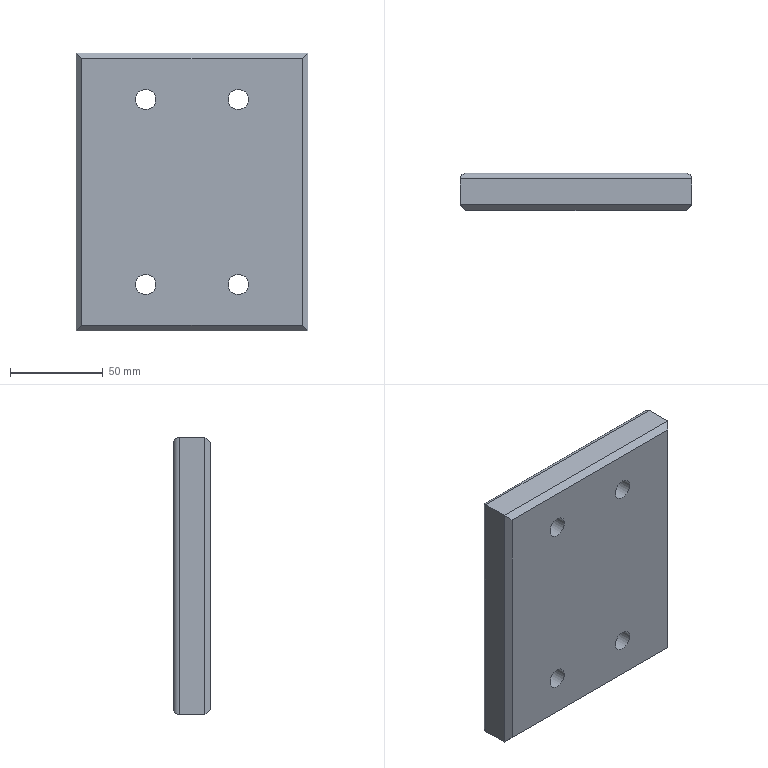Part | NX | features solid 2 | 1 solid | 26 faces | box 125 x 20 x 150 mm | volume 356923 mm3 | plane 14 | cylinder 12 | commonest cylinder face diameters 6 x4 11 x4 17.5 x4
STEP:
#1=CARTESIAN_POINT('',(-495.,793.,50.));
#2=VERTEX_POINT('',#1);
#3=CARTESIAN_POINT('',(-495.,807.,50.));
#4=VERTEX_POINT('',#3);
#5=CARTESIAN_POINT('',(-495.,790.,50.));
#6=DIRECTION('',(0.,1.,0.));
#7=VECTOR('',#6,1000.);
#8=LINE('',#5,#7);
#9=EDGE_CURVE('',#2,#4,#8,.T.);
#10=ORIENTED_EDGE('',*,*,#9,.F.);
#11=CARTESIAN_POINT('',(-620.,793.,50.));
#12=VERTEX_POINT('',#11);
#13=CARTESIAN_POINT('',(-620.,793.,50.));
#14=DIRECTION('',(-1.,0.,0.));
#15=VECTOR('',#14,1000.);
#16=LINE('',#13,#15);
#17=EDGE_CURVE('',#2,#12,#16,.T.);
#18=ORIENTED_EDGE('',*,*,#17,.T.);
#19=CARTESIAN_POINT('',(-620.,807.,50.));
#20=VERTEX_POINT('',#19);
#21=CARTESIAN_POINT('',(-620.,790.,50.));
#22=DIRECTION('',(0.,1.,0.));
#23=VECTOR('',#22,1000.);
#24=LINE('',#21,#23);
#25=EDGE_CURVE('',#12,#20,#24,.T.);
#26=ORIENTED_EDGE('',*,*,#25,.T.);
#27=CARTESIAN_POINT('',(-495.,807.,50.));
#28=DIRECTION('',(1.,0.,0.));
#29=VECTOR('',#28,1000.);
#30=LINE('',#27,#29);
#31=EDGE_CURVE('',#20,#4,#30,.T.);
#32=ORIENTED_EDGE('',*,*,#31,.T.);
#33=EDGE_LOOP('',(#10,#18,#26,#32));
#34=FACE_BOUND('',#33,.T.);
#35=CARTESIAN_POINT('',(-620.,790.,50.));
#36=DIRECTION('',(0.,0.,1.));
#37=DIRECTION('',(-1.,0.,0.));
#38=AXIS2_PLACEMENT_3D('',#35,#36,#37);
#39=PLANE('',#38);
#40=ADVANCED_FACE('',(#34),#39,.F.);
#41=CARTESIAN_POINT('',(-495.,793.,200.));
#42=VERTEX_POINT('',#41);
#43=CARTESIAN_POINT('',(-495.,807.,200.));
#44=VERTEX_POINT('',#43);
#45=CARTESIAN_POINT('',(-495.,790.,200.));
#46=DIRECTION('',(0.,1.,0.));
#47=VECTOR('',#46,1000.);
#48=LINE('',#45,#47);
#49=EDGE_CURVE('',#42,#44,#48,.T.);
#50=ORIENTED_EDGE('',*,*,#49,.F.);
#51=CARTESIAN_POINT('',(-495.,793.,50.));
#52=DIRECTION('',(0.,0.,-1.));
#53=VECTOR('',#52,1000.);
#54=LINE('',#51,#53);
#55=EDGE_CURVE('',#42,#2,#54,.T.);
#56=ORIENTED_EDGE('',*,*,#55,.T.);
#57=ORIENTED_EDGE('',*,*,#9,.T.);
#58=CARTESIAN_POINT('',(-495.,807.,200.));
#59=DIRECTION('',(0.,0.,1.));
#60=VECTOR('',#59,1000.);
#61=LINE('',#58,#60);
#62=EDGE_CURVE('',#4,#44,#61,.T.);
#63=ORIENTED_EDGE('',*,*,#62,.T.);
#64=EDGE_LOOP('',(#50,#56,#57,#63));
#65=FACE_BOUND('',#64,.T.);
#66=CARTESIAN_POINT('',(-495.,790.,50.));
#67=DIRECTION('',(-1.,0.,0.));
#68=DIRECTION('',(0.,-1.,0.));
#69=AXIS2_PLACEMENT_3D('',#66,#67,#68);
#70=PLANE('',#69);
#71=ADVANCED_FACE('',(#65),#70,.F.);
#72=CARTESIAN_POINT('',(-620.,793.,200.));
#73=VERTEX_POINT('',#72);
#74=CARTESIAN_POINT('',(-620.,807.,200.));
#75=VERTEX_POINT('',#74);
#76=CARTESIAN_POINT('',(-620.,790.,200.));
#77=DIRECTION('',(0.,1.,0.));
#78=VECTOR('',#77,1000.);
#79=LINE('',#76,#78);
#80=EDGE_CURVE('',#73,#75,#79,.T.);
#81=ORIENTED_EDGE('',*,*,#80,.F.);
#82=CARTESIAN_POINT('',(-495.,793.,200.));
#83=DIRECTION('',(1.,0.,0.));
#84=VECTOR('',#83,1000.);
#85=LINE('',#82,#84);
#86=EDGE_CURVE('',#73,#42,#85,.T.);
#87=ORIENTED_EDGE('',*,*,#86,.T.);
#88=ORIENTED_EDGE('',*,*,#49,.T.);
#89=CARTESIAN_POINT('',(-620.,807.,200.));
#90=DIRECTION('',(-1.,0.,0.));
#91=VECTOR('',#90,1000.);
#92=LINE('',#89,#91);
#93=EDGE_CURVE('',#44,#75,#92,.T.);
#94=ORIENTED_EDGE('',*,*,#93,.T.);
#95=EDGE_LOOP('',(#81,#87,#88,#94));
#96=FACE_BOUND('',#95,.T.);
#97=CARTESIAN_POINT('',(-495.,790.,200.));
#98=DIRECTION('',(0.,0.,-1.));
#99=DIRECTION('',(0.,-1.,0.));
#100=AXIS2_PLACEMENT_3D('',#97,#98,#99);
#101=PLANE('',#100);
#102=ADVANCED_FACE('',(#96),#101,.F.);
#103=ORIENTED_EDGE('',*,*,#25,.F.);
#104=CARTESIAN_POINT('',(-620.,793.,200.));
#105=DIRECTION('',(0.,0.,1.));
#106=VECTOR('',#105,1000.);
#107=LINE('',#104,#106);
#108=EDGE_CURVE('',#12,#73,#107,.T.);
#109=ORIENTED_EDGE('',*,*,#108,.T.);
#110=ORIENTED_EDGE('',*,*,#80,.T.);
#111=CARTESIAN_POINT('',(-620.,807.,50.));
#112=DIRECTION('',(0.,0.,-1.));
#113=VECTOR('',#112,1000.);
#114=LINE('',#111,#113);
#115=EDGE_CURVE('',#75,#20,#114,.T.);
#116=ORIENTED_EDGE('',*,*,#115,.T.);
#117=EDGE_LOOP('',(#103,#109,#110,#116));
#118=FACE_BOUND('',#117,.T.);
#119=CARTESIAN_POINT('',(-620.,790.,200.));
#120=DIRECTION('',(1.,0.,0.));
#121=DIRECTION('',(0.,0.,1.));
#122=AXIS2_PLACEMENT_3D('',#119,#120,#121);
#123=PLANE('',#122);
#124=ADVANCED_FACE('',(#118),#123,.F.);
#125=CARTESIAN_POINT('',(-498.,790.,53.));
#126=VERTEX_POINT('',#125);
#127=CARTESIAN_POINT('',(-498.,790.,197.));
#128=VERTEX_POINT('',#127);
#129=CARTESIAN_POINT('',(-498.,790.,50.));
#130=DIRECTION('',(0.,0.,1.));
#131=VECTOR('',#130,1000.);
#132=LINE('',#129,#131);
#133=EDGE_CURVE('',#126,#128,#132,.T.);
#134=ORIENTED_EDGE('',*,*,#133,.T.);
#135=CARTESIAN_POINT('',(-617.,790.,197.));
#136=VERTEX_POINT('',#135);
#137=CARTESIAN_POINT('',(-620.,790.,197.));
#138=DIRECTION('',(-1.,0.,0.));
#139=VECTOR('',#138,1000.);
#140=LINE('',#137,#139);
#141=EDGE_CURVE('',#128,#136,#140,.T.);
#142=ORIENTED_EDGE('',*,*,#141,.T.);
#143=CARTESIAN_POINT('',(-617.,790.,53.));
#144=VERTEX_POINT('',#143);
#145=CARTESIAN_POINT('',(-617.,790.,50.));
#146=DIRECTION('',(0.,0.,-1.));
#147=VECTOR('',#146,1000.);
#148=LINE('',#145,#147);
#149=EDGE_CURVE('',#136,#144,#148,.T.);
#150=ORIENTED_EDGE('',*,*,#149,.T.);
#151=CARTESIAN_POINT('',(-620.,790.,53.));
#152=DIRECTION('',(1.,0.,0.));
#153=VECTOR('',#152,1000.);
#154=LINE('',#151,#153);
#155=EDGE_CURVE('',#144,#126,#154,.T.);
#156=ORIENTED_EDGE('',*,*,#155,.T.);
#157=EDGE_LOOP('',(#134,#142,#150,#156));
#158=FACE_BOUND('',#157,.T.);
#159=CARTESIAN_POINT('',(-532.5,790.,169.5));
#160=VERTEX_POINT('',#159);
#161=CARTESIAN_POINT('',(-532.5,790.,175.));
#162=DIRECTION('',(0.,1.,0.));
#163=DIRECTION('',(0.,0.,-1.));
#164=AXIS2_PLACEMENT_3D('',#161,#162,#163);
#165=CIRCLE('',#164,5.5);
#166=EDGE_CURVE('',#160,#160,#165,.T.);
#167=ORIENTED_EDGE('',*,*,#166,.T.);
#168=EDGE_LOOP('',(#167));
#169=FACE_BOUND('',#168,.T.);
#170=CARTESIAN_POINT('',(-582.5,790.,169.5));
#171=VERTEX_POINT('',#170);
#172=CARTESIAN_POINT('',(-582.5,790.,175.));
#173=DIRECTION('',(0.,1.,0.));
#174=DIRECTION('',(0.,0.,-1.));
#175=AXIS2_PLACEMENT_3D('',#172,#173,#174);
#176=CIRCLE('',#175,5.5);
#177=EDGE_CURVE('',#171,#171,#176,.T.);
#178=ORIENTED_EDGE('',*,*,#177,.T.);
#179=EDGE_LOOP('',(#178));
#180=FACE_BOUND('',#179,.T.);
#181=CARTESIAN_POINT('',(-532.5,790.,69.5));
#182=VERTEX_POINT('',#181);
#183=CARTESIAN_POINT('',(-532.5,790.,75.));
#184=DIRECTION('',(0.,1.,0.));
#185=DIRECTION('',(0.,0.,-1.));
#186=AXIS2_PLACEMENT_3D('',#183,#184,#185);
#187=CIRCLE('',#186,5.5);
#188=EDGE_CURVE('',#182,#182,#187,.T.);
#189=ORIENTED_EDGE('',*,*,#188,.T.);
#190=EDGE_LOOP('',(#189));
#191=FACE_BOUND('',#190,.T.);
#192=CARTESIAN_POINT('',(-582.5,790.,69.5));
#193=VERTEX_POINT('',#192);
#194=CARTESIAN_POINT('',(-582.5,790.,75.));
#195=DIRECTION('',(0.,1.,0.));
#196=DIRECTION('',(0.,0.,-1.));
#197=AXIS2_PLACEMENT_3D('',#194,#195,#196);
#198=CIRCLE('',#197,5.5);
#199=EDGE_CURVE('',#193,#193,#198,.T.);
#200=ORIENTED_EDGE('',*,*,#199,.T.);
#201=EDGE_LOOP('',(#200));
#202=FACE_BOUND('',#201,.T.);
#203=CARTESIAN_POINT('',(-620.,790.,50.));
#204=DIRECTION('',(0.,1.,0.));
#205=DIRECTION('',(0.,0.,-1.));
#206=AXIS2_PLACEMENT_3D('',#203,#204,#205);
#207=PLANE('',#206);
#208=ADVANCED_FACE('',(#158,#169,#180,#191,#202),#207,.F.);
#209=CARTESIAN_POINT('',(-498.,810.,53.));
#210=VERTEX_POINT('',#209);
#211=CARTESIAN_POINT('',(-617.,810.,53.));
#212=VERTEX_POINT('',#211);
#213=CARTESIAN_POINT('',(-620.,810.,53.));
#214=DIRECTION('',(1.,0.,0.));
#215=VECTOR('',#214,1000.);
#216=LINE('',#213,#215);
#217=EDGE_CURVE('',#210,#212,#216,.F.);
#218=ORIENTED_EDGE('',*,*,#217,.T.);
#219=CARTESIAN_POINT('',(-617.,810.,197.));
#220=VERTEX_POINT('',#219);
#221=CARTESIAN_POINT('',(-617.,810.,200.));
#222=DIRECTION('',(0.,0.,-1.));
#223=VECTOR('',#222,1000.);
#224=LINE('',#221,#223);
#225=EDGE_CURVE('',#212,#220,#224,.F.);
#226=ORIENTED_EDGE('',*,*,#225,.T.);
#227=CARTESIAN_POINT('',(-498.,810.,197.));
#228=VERTEX_POINT('',#227);
#229=CARTESIAN_POINT('',(-495.,810.,197.));
#230=DIRECTION('',(-1.,0.,0.));
#231=VECTOR('',#230,1000.);
#232=LINE('',#229,#231);
#233=EDGE_CURVE('',#220,#228,#232,.F.);
#234=ORIENTED_EDGE('',*,*,#233,.T.);
#235=CARTESIAN_POINT('',(-498.,810.,50.));
#236=DIRECTION('',(0.,0.,1.));
#237=VECTOR('',#236,1000.);
#238=LINE('',#235,#237);
#239=EDGE_CURVE('',#228,#210,#238,.F.);
#240=ORIENTED_EDGE('',*,*,#239,.T.);
#241=EDGE_LOOP('',(#218,#226,#234,#240));
#242=FACE_BOUND('',#241,.T.);
#243=CARTESIAN_POINT('',(-532.5,810.,183.75));
#244=VERTEX_POINT('',#243);
#245=CARTESIAN_POINT('',(-532.5,810.,175.));
#246=DIRECTION('',(0.,-1.,0.));
#247=DIRECTION('',(0.,0.,1.));
#248=AXIS2_PLACEMENT_3D('',#245,#246,#247);
#249=CIRCLE('',#248,8.75);
#250=EDGE_CURVE('',#244,#244,#249,.T.);
#251=ORIENTED_EDGE('',*,*,#250,.T.);
#252=EDGE_LOOP('',(#251));
#253=FACE_BOUND('',#252,.T.);
#254=CARTESIAN_POINT('',(-582.5,810.,183.75));
#255=VERTEX_POINT('',#254);
#256=CARTESIAN_POINT('',(-582.5,810.,175.));
#257=DIRECTION('',(0.,-1.,0.));
#258=DIRECTION('',(0.,0.,1.));
#259=AXIS2_PLACEMENT_3D('',#256,#257,#258);
#260=CIRCLE('',#259,8.75);
#261=EDGE_CURVE('',#255,#255,#260,.T.);
#262=ORIENTED_EDGE('',*,*,#261,.T.);
#263=EDGE_LOOP('',(#262));
#264=FACE_BOUND('',#263,.T.);
#265=CARTESIAN_POINT('',(-532.5,810.,83.75));
#266=VERTEX_POINT('',#265);
#267=CARTESIAN_POINT('',(-532.5,810.,75.));
#268=DIRECTION('',(0.,-1.,0.));
#269=DIRECTION('',(0.,0.,1.));
#270=AXIS2_PLACEMENT_3D('',#267,#268,#269);
#271=CIRCLE('',#270,8.75);
#272=EDGE_CURVE('',#266,#266,#271,.T.);
#273=ORIENTED_EDGE('',*,*,#272,.T.);
#274=EDGE_LOOP('',(#273));
#275=FACE_BOUND('',#274,.T.);
#276=CARTESIAN_POINT('',(-582.5,810.,83.75));
#277=VERTEX_POINT('',#276);
#278=CARTESIAN_POINT('',(-582.5,810.,75.));
#279=DIRECTION('',(0.,-1.,0.));
#280=DIRECTION('',(0.,0.,1.));
#281=AXIS2_PLACEMENT_3D('',#278,#279,#280);
#282=CIRCLE('',#281,8.75);
#283=EDGE_CURVE('',#277,#277,#282,.T.);
#284=ORIENTED_EDGE('',*,*,#283,.T.);
#285=EDGE_LOOP('',(#284));
#286=FACE_BOUND('',#285,.T.);
#287=CARTESIAN_POINT('',(-620.,810.,50.));
#288=DIRECTION('',(0.,1.,0.));
#289=DIRECTION('',(0.,0.,-1.));
#290=AXIS2_PLACEMENT_3D('',#287,#288,#289);
#291=PLANE('',#290);
#292=ADVANCED_FACE('',(#242,#253,#264,#275,#286),#291,.T.);
#293=CARTESIAN_POINT('',(-582.5,798.,80.5));
#294=VERTEX_POINT('',#293);
#295=CARTESIAN_POINT('',(-582.5,798.,75.));
#296=DIRECTION('',(0.,-1.,0.));
#297=DIRECTION('',(0.,0.,1.));
#298=AXIS2_PLACEMENT_3D('',#295,#296,#297);
#299=CIRCLE('',#298,5.5);
#300=EDGE_CURVE('',#294,#294,#299,.T.);
#301=ORIENTED_EDGE('',*,*,#300,.F.);
#302=EDGE_LOOP('',(#301));
#303=FACE_BOUND('',#302,.T.);
#304=ORIENTED_EDGE('',*,*,#199,.F.);
#305=EDGE_LOOP('',(#304));
#306=FACE_BOUND('',#305,.T.);
#307=CARTESIAN_POINT('',(-582.5,760.,75.));
#308=DIRECTION('',(0.,-1.,0.));
#309=DIRECTION('',(0.,0.,1.));
#310=AXIS2_PLACEMENT_3D('',#307,#308,#309);
#311=CYLINDRICAL_SURFACE('',#310,5.5);
#312=ADVANCED_FACE('',(#303,#306),#311,.F.);
#313=ORIENTED_EDGE('',*,*,#300,.T.);
#314=EDGE_LOOP('',(#313));
#315=FACE_BOUND('',#314,.T.);
#316=CARTESIAN_POINT('',(-582.5,798.,83.75));
#317=VERTEX_POINT('',#316);
#318=CARTESIAN_POINT('',(-582.5,798.,75.));
#319=DIRECTION('',(0.,-1.,0.));
#320=DIRECTION('',(0.,0.,1.));
#321=AXIS2_PLACEMENT_3D('',#318,#319,#320);
#322=CIRCLE('',#321,8.75);
#323=EDGE_CURVE('',#317,#317,#322,.T.);
#324=ORIENTED_EDGE('',*,*,#323,.F.);
#325=EDGE_LOOP('',(#324));
#326=FACE_BOUND('',#325,.T.);
#327=CARTESIAN_POINT('',(-582.5,798.,75.));
#328=DIRECTION('',(0.,-1.,0.));
#329=DIRECTION('',(0.,0.,1.));
#330=AXIS2_PLACEMENT_3D('',#327,#328,#329);
#331=PLANE('',#330);
#332=ADVANCED_FACE('',(#315,#326),#331,.F.);
#333=ORIENTED_EDGE('',*,*,#323,.T.);
#334=EDGE_LOOP('',(#333));
#335=FACE_BOUND('',#334,.T.);
#336=ORIENTED_EDGE('',*,*,#283,.F.);
#337=EDGE_LOOP('',(#336));
#338=FACE_BOUND('',#337,.T.);
#339=CARTESIAN_POINT('',(-582.5,810.,75.));
#340=DIRECTION('',(0.,-1.,0.));
#341=DIRECTION('',(0.,0.,1.));
#342=AXIS2_PLACEMENT_3D('',#339,#340,#341);
#343=CYLINDRICAL_SURFACE('',#342,8.75);
#344=ADVANCED_FACE('',(#335,#338),#343,.F.);
#345=CARTESIAN_POINT('',(-532.5,798.,80.5));
#346=VERTEX_POINT('',#345);
#347=CARTESIAN_POINT('',(-532.5,798.,75.));
#348=DIRECTION('',(0.,-1.,0.));
#349=DIRECTION('',(0.,0.,1.));
#350=AXIS2_PLACEMENT_3D('',#347,#348,#349);
#351=CIRCLE('',#350,5.5);
#352=EDGE_CURVE('',#346,#346,#351,.T.);
#353=ORIENTED_EDGE('',*,*,#352,.F.);
#354=EDGE_LOOP('',(#353));
#355=FACE_BOUND('',#354,.T.);
#356=ORIENTED_EDGE('',*,*,#188,.F.);
#357=EDGE_LOOP('',(#356));
#358=FACE_BOUND('',#357,.T.);
#359=CARTESIAN_POINT('',(-532.5,760.,75.));
#360=DIRECTION('',(0.,-1.,0.));
#361=DIRECTION('',(0.,0.,1.));
#362=AXIS2_PLACEMENT_3D('',#359,#360,#361);
#363=CYLINDRICAL_SURFACE('',#362,5.5);
#364=ADVANCED_FACE('',(#355,#358),#363,.F.);
#365=ORIENTED_EDGE('',*,*,#352,.T.);
#366=EDGE_LOOP('',(#365));
#367=FACE_BOUND('',#366,.T.);
#368=CARTESIAN_POINT('',(-532.5,798.,83.75));
#369=VERTEX_POINT('',#368);
#370=CARTESIAN_POINT('',(-532.5,798.,75.));
#371=DIRECTION('',(0.,-1.,0.));
#372=DIRECTION('',(0.,0.,1.));
#373=AXIS2_PLACEMENT_3D('',#370,#371,#372);
#374=CIRCLE('',#373,8.75);
#375=EDGE_CURVE('',#369,#369,#374,.T.);
#376=ORIENTED_EDGE('',*,*,#375,.F.);
#377=EDGE_LOOP('',(#376));
#378=FACE_BOUND('',#377,.T.);
#379=CARTESIAN_POINT('',(-532.5,798.,75.));
#380=DIRECTION('',(0.,-1.,0.));
#381=DIRECTION('',(0.,0.,1.));
#382=AXIS2_PLACEMENT_3D('',#379,#380,#381);
#383=PLANE('',#382);
#384=ADVANCED_FACE('',(#367,#378),#383,.F.);
#385=ORIENTED_EDGE('',*,*,#375,.T.);
#386=EDGE_LOOP('',(#385));
#387=FACE_BOUND('',#386,.T.);
#388=ORIENTED_EDGE('',*,*,#272,.F.);
#389=EDGE_LOOP('',(#388));
#390=FACE_BOUND('',#389,.T.);
#391=CARTESIAN_POINT('',(-532.5,810.,75.));
#392=DIRECTION('',(0.,-1.,0.));
#393=DIRECTION('',(0.,0.,1.));
#394=AXIS2_PLACEMENT_3D('',#391,#392,#393);
#395=CYLINDRICAL_SURFACE('',#394,8.75);
#396=ADVANCED_FACE('',(#387,#390),#395,.F.);
#397=CARTESIAN_POINT('',(-582.5,798.,180.5));
#398=VERTEX_POINT('',#397);
#399=CARTESIAN_POINT('',(-582.5,798.,175.));
#400=DIRECTION('',(0.,-1.,0.));
#401=DIRECTION('',(0.,0.,1.));
#402=AXIS2_PLACEMENT_3D('',#399,#400,#401);
#403=CIRCLE('',#402,5.5);
#404=EDGE_CURVE('',#398,#398,#403,.T.);
#405=ORIENTED_EDGE('',*,*,#404,.F.);
#406=EDGE_LOOP('',(#405));
#407=FACE_BOUND('',#406,.T.);
#408=ORIENTED_EDGE('',*,*,#177,.F.);
#409=EDGE_LOOP('',(#408));
#410=FACE_BOUND('',#409,.T.);
#411=CARTESIAN_POINT('',(-582.5,760.,175.));
#412=DIRECTION('',(0.,-1.,0.));
#413=DIRECTION('',(0.,0.,1.));
#414=AXIS2_PLACEMENT_3D('',#411,#412,#413);
#415=CYLINDRICAL_SURFACE('',#414,5.5);
#416=ADVANCED_FACE('',(#407,#410),#415,.F.);
#417=ORIENTED_EDGE('',*,*,#404,.T.);
#418=EDGE_LOOP('',(#417));
#419=FACE_BOUND('',#418,.T.);
#420=CARTESIAN_POINT('',(-582.5,798.,183.75));
#421=VERTEX_POINT('',#420);
#422=CARTESIAN_POINT('',(-582.5,798.,175.));
#423=DIRECTION('',(0.,-1.,0.));
#424=DIRECTION('',(0.,0.,1.));
#425=AXIS2_PLACEMENT_3D('',#422,#423,#424);
#426=CIRCLE('',#425,8.75);
#427=EDGE_CURVE('',#421,#421,#426,.T.);
#428=ORIENTED_EDGE('',*,*,#427,.F.);
#429=EDGE_LOOP('',(#428));
#430=FACE_BOUND('',#429,.T.);
#431=CARTESIAN_POINT('',(-582.5,798.,175.));
#432=DIRECTION('',(0.,-1.,0.));
#433=DIRECTION('',(0.,0.,1.));
#434=AXIS2_PLACEMENT_3D('',#431,#432,#433);
#435=PLANE('',#434);
#436=ADVANCED_FACE('',(#419,#430),#435,.F.);
#437=ORIENTED_EDGE('',*,*,#427,.T.);
#438=EDGE_LOOP('',(#437));
#439=FACE_BOUND('',#438,.T.);
#440=ORIENTED_EDGE('',*,*,#261,.F.);
#441=EDGE_LOOP('',(#440));
#442=FACE_BOUND('',#441,.T.);
#443=CARTESIAN_POINT('',(-582.5,810.,175.));
#444=DIRECTION('',(0.,-1.,0.));
#445=DIRECTION('',(0.,0.,1.));
#446=AXIS2_PLACEMENT_3D('',#443,#444,#445);
#447=CYLINDRICAL_SURFACE('',#446,8.75);
#448=ADVANCED_FACE('',(#439,#442),#447,.F.);
#449=CARTESIAN_POINT('',(-532.5,798.,180.5));
#450=VERTEX_POINT('',#449);
#451=CARTESIAN_POINT('',(-532.5,798.,175.));
#452=DIRECTION('',(0.,-1.,0.));
#453=DIRECTION('',(0.,0.,1.));
#454=AXIS2_PLACEMENT_3D('',#451,#452,#453);
#455=CIRCLE('',#454,5.5);
#456=EDGE_CURVE('',#450,#450,#455,.T.);
#457=ORIENTED_EDGE('',*,*,#456,.F.);
#458=EDGE_LOOP('',(#457));
#459=FACE_BOUND('',#458,.T.);
#460=ORIENTED_EDGE('',*,*,#166,.F.);
#461=EDGE_LOOP('',(#460));
#462=FACE_BOUND('',#461,.T.);
#463=CARTESIAN_POINT('',(-532.5,760.,175.));
#464=DIRECTION('',(0.,-1.,0.));
#465=DIRECTION('',(0.,0.,1.));
#466=AXIS2_PLACEMENT_3D('',#463,#464,#465);
#467=CYLINDRICAL_SURFACE('',#466,5.5);
#468=ADVANCED_FACE('',(#459,#462),#467,.F.);
#469=ORIENTED_EDGE('',*,*,#456,.T.);
#470=EDGE_LOOP('',(#469));
#471=FACE_BOUND('',#470,.T.);
#472=CARTESIAN_POINT('',(-532.5,798.,183.75));
#473=VERTEX_POINT('',#472);
#474=CARTESIAN_POINT('',(-532.5,798.,175.));
#475=DIRECTION('',(0.,-1.,0.));
#476=DIRECTION('',(0.,0.,1.));
#477=AXIS2_PLACEMENT_3D('',#474,#475,#476);
#478=CIRCLE('',#477,8.75);
#479=EDGE_CURVE('',#473,#473,#478,.T.);
#480=ORIENTED_EDGE('',*,*,#479,.F.);
#481=EDGE_LOOP('',(#480));
#482=FACE_BOUND('',#481,.T.);
#483=CARTESIAN_POINT('',(-532.5,798.,175.));
#484=DIRECTION('',(0.,-1.,0.));
#485=DIRECTION('',(0.,0.,1.));
#486=AXIS2_PLACEMENT_3D('',#483,#484,#485);
#487=PLANE('',#486);
#488=ADVANCED_FACE('',(#471,#482),#487,.F.);
#489=ORIENTED_EDGE('',*,*,#479,.T.);
#490=EDGE_LOOP('',(#489));
#491=FACE_BOUND('',#490,.T.);
#492=ORIENTED_EDGE('',*,*,#250,.F.);
#493=EDGE_LOOP('',(#492));
#494=FACE_BOUND('',#493,.T.);
#495=CARTESIAN_POINT('',(-532.5,810.,175.));
#496=DIRECTION('',(0.,-1.,0.));
#497=DIRECTION('',(0.,0.,1.));
#498=AXIS2_PLACEMENT_3D('',#495,#496,#497);
#499=CYLINDRICAL_SURFACE('',#498,8.75);
#500=ADVANCED_FACE('',(#491,#494),#499,.F.);
#501=CARTESIAN_POINT('',(-498.,807.,53.));
#502=DIRECTION('',(-0.7071,0.,-0.7071));
#503=DIRECTION('',(-0.7071,0.,0.7071));
#504=AXIS2_PLACEMENT_3D('',#501,#502,#503);
#505=ELLIPSE('',#504,4.243,3.);
#506=EDGE_CURVE('',#210,#4,#505,.T.);
#507=ORIENTED_EDGE('',*,*,#506,.F.);
#508=ORIENTED_EDGE('',*,*,#239,.F.);
#509=CARTESIAN_POINT('',(-498.,807.,197.));
#510=DIRECTION('',(0.7071,0.,-0.7071));
#511=DIRECTION('',(-0.7071,0.,-0.7071));
#512=AXIS2_PLACEMENT_3D('',#509,#510,#511);
#513=ELLIPSE('',#512,4.243,3.);
#514=EDGE_CURVE('',#44,#228,#513,.F.);
#515=ORIENTED_EDGE('',*,*,#514,.F.);
#516=ORIENTED_EDGE('',*,*,#62,.F.);
#517=EDGE_LOOP('',(#507,#508,#515,#516));
#518=FACE_BOUND('',#517,.T.);
#519=CARTESIAN_POINT('',(-498.,807.,50.));
#520=DIRECTION('',(0.,0.,-1.));
#521=DIRECTION('',(0.,-1.,0.));
#522=AXIS2_PLACEMENT_3D('',#519,#520,#521);
#523=CYLINDRICAL_SURFACE('',#522,3.);
#524=ADVANCED_FACE('',(#518),#523,.T.);
#525=ORIENTED_EDGE('',*,*,#514,.T.);
#526=ORIENTED_EDGE('',*,*,#233,.F.);
#527=CARTESIAN_POINT('',(-617.,807.,197.));
#528=DIRECTION('',(0.7071,0.,0.7071));
#529=DIRECTION('',(0.7071,0.,-0.7071));
#530=AXIS2_PLACEMENT_3D('',#527,#528,#529);
#531=ELLIPSE('',#530,4.243,3.);
#532=EDGE_CURVE('',#75,#220,#531,.F.);
#533=ORIENTED_EDGE('',*,*,#532,.F.);
#534=ORIENTED_EDGE('',*,*,#93,.F.);
#535=EDGE_LOOP('',(#525,#526,#533,#534));
#536=FACE_BOUND('',#535,.T.);
#537=CARTESIAN_POINT('',(-495.,807.,197.));
#538=DIRECTION('',(1.,0.,0.));
#539=DIRECTION('',(0.,1.,0.));
#540=AXIS2_PLACEMENT_3D('',#537,#538,#539);
#541=CYLINDRICAL_SURFACE('',#540,3.);
#542=ADVANCED_FACE('',(#536),#541,.T.);
#543=ORIENTED_EDGE('',*,*,#506,.T.);
#544=ORIENTED_EDGE('',*,*,#31,.F.);
#545=CARTESIAN_POINT('',(-617.,807.,53.));
#546=DIRECTION('',(-0.7071,0.,0.7071));
#547=DIRECTION('',(-0.7071,0.,-0.7071));
#548=AXIS2_PLACEMENT_3D('',#545,#546,#547);
#549=ELLIPSE('',#548,4.243,3.);
#550=EDGE_CURVE('',#212,#20,#549,.T.);
#551=ORIENTED_EDGE('',*,*,#550,.F.);
#552=ORIENTED_EDGE('',*,*,#217,.F.);
#553=EDGE_LOOP('',(#543,#544,#551,#552));
#554=FACE_BOUND('',#553,.T.);
#555=CARTESIAN_POINT('',(-620.,807.,53.));
#556=DIRECTION('',(-1.,0.,0.));
#557=DIRECTION('',(0.,0.,-1.));
#558=AXIS2_PLACEMENT_3D('',#555,#556,#557);
#559=CYLINDRICAL_SURFACE('',#558,3.);
#560=ADVANCED_FACE('',(#554),#559,.T.);
#561=ORIENTED_EDGE('',*,*,#532,.T.);
#562=ORIENTED_EDGE('',*,*,#225,.F.);
#563=ORIENTED_EDGE('',*,*,#550,.T.);
#564=ORIENTED_EDGE('',*,*,#115,.F.);
#565=EDGE_LOOP('',(#561,#562,#563,#564));
#566=FACE_BOUND('',#565,.T.);
#567=CARTESIAN_POINT('',(-617.,807.,200.));
#568=DIRECTION('',(0.,0.,1.));
#569=DIRECTION('',(-1.,0.,0.));
#570=AXIS2_PLACEMENT_3D('',#567,#568,#569);
#571=CYLINDRICAL_SURFACE('',#570,3.);
#572=ADVANCED_FACE('',(#566),#571,.T.);
#573=CARTESIAN_POINT('',(-618.,791.,52.));
#574=DIRECTION('',(0.5774,-0.5774,0.5774));
#575=VECTOR('',#574,1000.);
#576=LINE('',#573,#575);
#577=EDGE_CURVE('',#12,#144,#576,.T.);
#578=ORIENTED_EDGE('',*,*,#577,.F.);
#579=ORIENTED_EDGE('',*,*,#17,.F.);
#580=CARTESIAN_POINT('',(-538.667,749.333,93.667));
#581=DIRECTION('',(-0.5774,-0.5774,0.5774));
#582=VECTOR('',#581,1000.);
#583=LINE('',#580,#582);
#584=EDGE_CURVE('',#126,#2,#583,.F.);
#585=ORIENTED_EDGE('',*,*,#584,.F.);
#586=ORIENTED_EDGE('',*,*,#155,.F.);
#587=EDGE_LOOP('',(#578,#579,#585,#586));
#588=FACE_BOUND('',#587,.T.);
#589=CARTESIAN_POINT('',(-620.,790.,53.));
#590=DIRECTION('',(0.,0.7071,0.7071));
#591=DIRECTION('',(0.,0.7071,-0.7071));
#592=AXIS2_PLACEMENT_3D('',#589,#590,#591);
#593=PLANE('',#592);
#594=ADVANCED_FACE('',(#588),#593,.F.);
#595=ORIENTED_EDGE('',*,*,#584,.T.);
#596=ORIENTED_EDGE('',*,*,#55,.F.);
#597=CARTESIAN_POINT('',(-547.,741.,148.));
#598=DIRECTION('',(-0.5774,-0.5774,-0.5774));
#599=VECTOR('',#598,1000.);
#600=LINE('',#597,#599);
#601=EDGE_CURVE('',#128,#42,#600,.F.);
#602=ORIENTED_EDGE('',*,*,#601,.F.);
#603=ORIENTED_EDGE('',*,*,#133,.F.);
#604=EDGE_LOOP('',(#595,#596,#602,#603));
#605=FACE_BOUND('',#604,.T.);
#606=CARTESIAN_POINT('',(-498.,790.,50.));
#607=DIRECTION('',(-0.7071,0.7071,0.));
#608=DIRECTION('',(-0.7071,-0.7071,0.));
#609=AXIS2_PLACEMENT_3D('',#606,#607,#608);
#610=PLANE('',#609);
#611=ADVANCED_FACE('',(#605),#610,.F.);
#612=ORIENTED_EDGE('',*,*,#577,.T.);
#613=ORIENTED_EDGE('',*,*,#149,.F.);
#614=CARTESIAN_POINT('',(-568.,741.,148.));
#615=DIRECTION('',(-0.5774,0.5774,0.5774));
#616=VECTOR('',#615,1000.);
#617=LINE('',#614,#616);
#618=EDGE_CURVE('',#73,#136,#617,.F.);
#619=ORIENTED_EDGE('',*,*,#618,.F.);
#620=ORIENTED_EDGE('',*,*,#108,.F.);
#621=EDGE_LOOP('',(#612,#613,#619,#620));
#622=FACE_BOUND('',#621,.T.);
#623=CARTESIAN_POINT('',(-617.,790.,50.));
#624=DIRECTION('',(0.7071,0.7071,0.));
#625=DIRECTION('',(-0.7071,0.7071,0.));
#626=AXIS2_PLACEMENT_3D('',#623,#624,#625);
#627=PLANE('',#626);
#628=ADVANCED_FACE('',(#622),#627,.F.);
#629=ORIENTED_EDGE('',*,*,#601,.T.);
#630=ORIENTED_EDGE('',*,*,#86,.F.);
#631=ORIENTED_EDGE('',*,*,#618,.T.);
#632=ORIENTED_EDGE('',*,*,#141,.F.);
#633=EDGE_LOOP('',(#629,#630,#631,#632));
#634=FACE_BOUND('',#633,.T.);
#635=CARTESIAN_POINT('',(-620.,790.,197.));
#636=DIRECTION('',(0.,0.7071,-0.7071));
#637=DIRECTION('',(0.,-0.7071,-0.7071));
#638=AXIS2_PLACEMENT_3D('',#635,#636,#637);
#639=PLANE('',#638);
#640=ADVANCED_FACE('',(#634),#639,.F.);
#641=CLOSED_SHELL('',(#40,#71,#102,#124,#208,#292,#312,#332,#344,#364,#384,#396,#416,#436,#448,#468,#488,#500,#524,#542,#560,#572,#594,#611,#628,#640));
#642=MANIFOLD_SOLID_BREP('',#641);
#643=(LENGTH_UNIT()NAMED_UNIT(*)SI_UNIT(.MILLI.,.METRE.));
#644=UNCERTAINTY_MEASURE_WITH_UNIT(LENGTH_MEASURE(0.00001),#643,'','');
#645=(NAMED_UNIT(*)PLANE_ANGLE_UNIT()SI_UNIT($,.RADIAN.));
#646=(NAMED_UNIT(*)SI_UNIT($,.STERADIAN.)SOLID_ANGLE_UNIT());
#647=(GEOMETRIC_REPRESENTATION_CONTEXT(3)GLOBAL_UNCERTAINTY_ASSIGNED_CONTEXT((#644))GLOBAL_UNIT_ASSIGNED_CONTEXT((#643,#645,#646))REPRESENTATION_CONTEXT('',''));
#648=ADVANCED_BREP_SHAPE_REPRESENTATION('',(#642),#647);